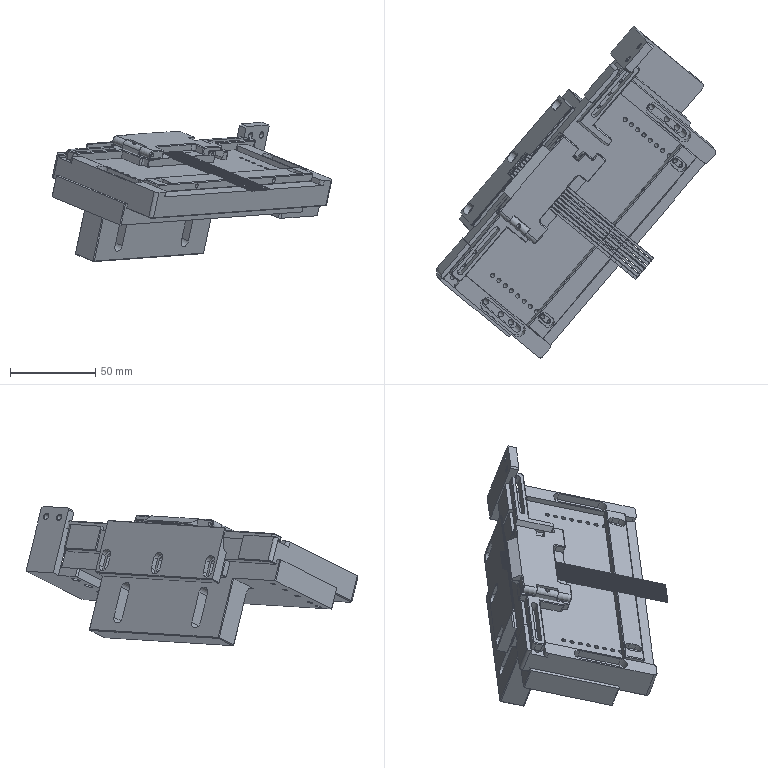Part | SolidWorks | 9 solids | 1470 faces | box 164.031 x 194.596 x 81.627 mm | volume 348427 mm3 | plane 711 | cylinder 629 | spline 96 | cone 34 | commonest cylinder face diameters 0.1 x98 2.5 x74 0.16 x64 0.223 x48 0.26 x48 0.5 x48